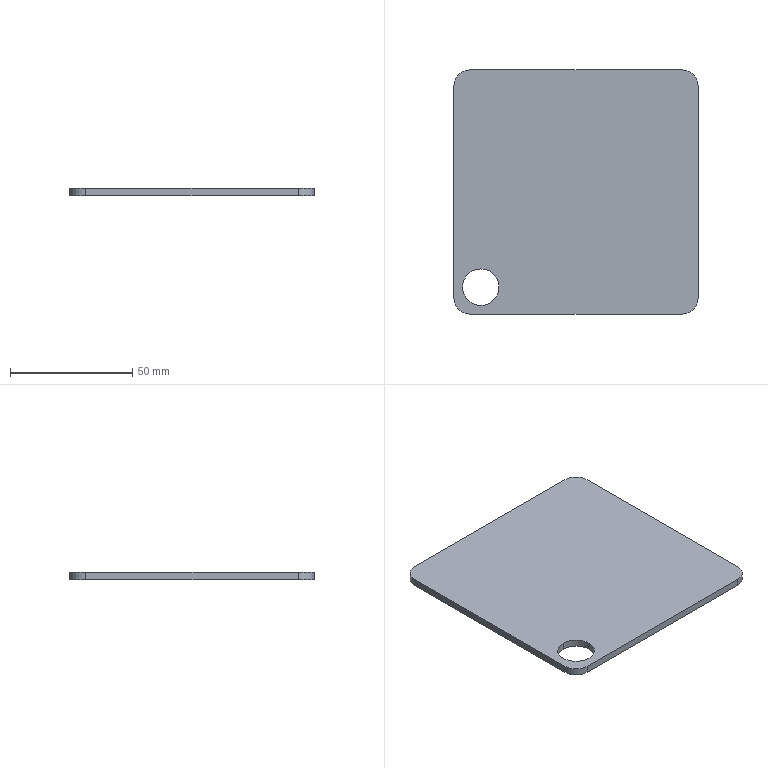Part | STEP file | [14] | 1 solid | 12 faces | box 100 x 100 x 3 mm | volume 29364 mm3 | cylinder 6 | plane 6 | commonest cylinder face diameters 12.8 x4 15 x2
STEP:
#1=CARTESIAN_POINT('',(0.,0.,0.));
#2=DIRECTION('',(0.,0.,1.));
#3=DIRECTION('',(1.,0.,0.));
#4=AXIS2_PLACEMENT_3D('',#1,#2,#3);
#5=CARTESIAN_POINT('',(11.,3.5,0.));
#6=VERTEX_POINT('',#5);
#7=CARTESIAN_POINT('',(11.,3.5,3.));
#8=VERTEX_POINT('',#7);
#9=CARTESIAN_POINT('',(11.,3.5,0.));
#10=DIRECTION('',(0.,0.,1.));
#11=VECTOR('',#10,1.);
#12=LINE('',#9,#11);
#13=CARTESIAN_POINT('',(11.,11.,0.));
#14=DIRECTION('',(0.,0.,1.));
#15=DIRECTION('',(0.,-1.,0.));
#16=AXIS2_PLACEMENT_3D('',#13,#14,#15);
#17=CYLINDRICAL_SURFACE('',#16,7.5);
#18=CARTESIAN_POINT('',(6.283,0.));
#19=DIRECTION('',(0.,1.));
#20=VECTOR('',#19,1.);
#21=LINE('',#18,#20);
#22=(GEOMETRIC_REPRESENTATION_CONTEXT(2)PARAMETRIC_REPRESENTATION_CONTEXT()REPRESENTATION_CONTEXT('',''));
#23=DEFINITIONAL_REPRESENTATION('',(#21),#22);
#24=PCURVE('',#17,#23);
#25=CARTESIAN_POINT('',(11.,11.,0.));
#26=DIRECTION('',(0.,0.,1.));
#27=DIRECTION('',(0.,-1.,0.));
#28=AXIS2_PLACEMENT_3D('',#25,#26,#27);
#29=CYLINDRICAL_SURFACE('',#28,7.5);
#30=CARTESIAN_POINT('',(0.,0.));
#31=DIRECTION('',(0.,1.));
#32=VECTOR('',#31,1.);
#33=LINE('',#30,#32);
#34=(GEOMETRIC_REPRESENTATION_CONTEXT(2)PARAMETRIC_REPRESENTATION_CONTEXT()REPRESENTATION_CONTEXT('',''));
#35=DEFINITIONAL_REPRESENTATION('',(#33),#34);
#36=PCURVE('',#29,#35);
#37=SURFACE_CURVE('',#12,(#24,#36),.PCURVE_S1.);
#38=EDGE_CURVE('',#6,#8,#37,.T.);
#39=ORIENTED_EDGE('',*,*,#38,.T.);
#40=CARTESIAN_POINT('',(11.,18.5,3.));
#41=VERTEX_POINT('',#40);
#42=CARTESIAN_POINT('',(11.,11.,3.));
#43=DIRECTION('',(0.,0.,-1.));
#44=DIRECTION('',(0.,1.,0.));
#45=AXIS2_PLACEMENT_3D('',#42,#43,#44);
#46=CIRCLE('',#45,7.5);
#47=CARTESIAN_POINT('',(9.425,3.));
#48=DIRECTION('',(-1.,0.));
#49=VECTOR('',#48,1.);
#50=LINE('',#47,#49);
#51=(GEOMETRIC_REPRESENTATION_CONTEXT(2)PARAMETRIC_REPRESENTATION_CONTEXT()REPRESENTATION_CONTEXT('',''));
#52=DEFINITIONAL_REPRESENTATION('',(#50),#51);
#53=PCURVE('',#17,#52);
#54=CARTESIAN_POINT('',(50.,50.,3.));
#55=DIRECTION('',(0.,0.,1.));
#56=DIRECTION('',(-1.,0.,0.));
#57=AXIS2_PLACEMENT_3D('',#54,#55,#56);
#58=PLANE('',#57);
#59=CARTESIAN_POINT('',(39.,31.5));
#60=CARTESIAN_POINT('',(26.01,31.5));
#61=CARTESIAN_POINT('',(32.505,42.75));
#62=CARTESIAN_POINT('',(39.,54.));
#63=CARTESIAN_POINT('',(45.495,42.75));
#64=CARTESIAN_POINT('',(51.99,31.5));
#65=CARTESIAN_POINT('',(39.,31.5));
#66=(BOUNDED_CURVE()B_SPLINE_CURVE(2,(#59,#60,#61,#62,#63,#64,#65),.UNSPECIFIED.,.T.,.F.)B_SPLINE_CURVE_WITH_KNOTS((1,2,2,2,2,1),(-2.094,0.,2.094,4.189,6.283,8.378),.UNSPECIFIED.)CURVE()GEOMETRIC_REPRESENTATION_ITEM()RATIONAL_B_SPLINE_CURVE((1.,0.5,1.,0.5,1.,0.5,1.))REPRESENTATION_ITEM(''));
#67=(GEOMETRIC_REPRESENTATION_CONTEXT(2)PARAMETRIC_REPRESENTATION_CONTEXT()REPRESENTATION_CONTEXT('',''));
#68=DEFINITIONAL_REPRESENTATION('',(#66),#67);
#69=PCURVE('',#58,#68);
#70=SURFACE_CURVE('',#46,(#53,#69),.PCURVE_S1.);
#71=EDGE_CURVE('',#8,#41,#70,.T.);
#72=ORIENTED_EDGE('',*,*,#71,.T.);
#73=CARTESIAN_POINT('',(11.,18.5,0.));
#74=VERTEX_POINT('',#73);
#75=CARTESIAN_POINT('',(11.,18.5,0.));
#76=DIRECTION('',(0.,0.,1.));
#77=VECTOR('',#76,1.);
#78=LINE('',#75,#77);
#79=CARTESIAN_POINT('',(3.142,0.));
#80=DIRECTION('',(0.,1.));
#81=VECTOR('',#80,1.);
#82=LINE('',#79,#81);
#83=(GEOMETRIC_REPRESENTATION_CONTEXT(2)PARAMETRIC_REPRESENTATION_CONTEXT()REPRESENTATION_CONTEXT('',''));
#84=DEFINITIONAL_REPRESENTATION('',(#82),#83);
#85=PCURVE('',#17,#84);
#86=CARTESIAN_POINT('',(3.142,0.));
#87=DIRECTION('',(0.,1.));
#88=VECTOR('',#87,1.);
#89=LINE('',#86,#88);
#90=(GEOMETRIC_REPRESENTATION_CONTEXT(2)PARAMETRIC_REPRESENTATION_CONTEXT()REPRESENTATION_CONTEXT('',''));
#91=DEFINITIONAL_REPRESENTATION('',(#89),#90);
#92=PCURVE('',#29,#91);
#93=SURFACE_CURVE('',#78,(#85,#92),.PCURVE_S1.);
#94=EDGE_CURVE('',#74,#41,#93,.T.);
#95=ORIENTED_EDGE('',*,*,#94,.F.);
#96=CARTESIAN_POINT('',(11.,11.,0.));
#97=DIRECTION('',(0.,0.,1.));
#98=DIRECTION('',(0.,-1.,0.));
#99=AXIS2_PLACEMENT_3D('',#96,#97,#98);
#100=CIRCLE('',#99,7.5);
#101=CARTESIAN_POINT('',(0.,0.));
#102=DIRECTION('',(1.,0.));
#103=VECTOR('',#102,1.);
#104=LINE('',#101,#103);
#105=(GEOMETRIC_REPRESENTATION_CONTEXT(2)PARAMETRIC_REPRESENTATION_CONTEXT()REPRESENTATION_CONTEXT('',''));
#106=DEFINITIONAL_REPRESENTATION('',(#104),#105);
#107=PCURVE('',#17,#106);
#108=CARTESIAN_POINT('',(50.,50.,0.));
#109=DIRECTION('',(0.,0.,-1.));
#110=DIRECTION('',(1.,0.,0.));
#111=AXIS2_PLACEMENT_3D('',#108,#109,#110);
#112=PLANE('',#111);
#113=CARTESIAN_POINT('',(-39.,46.5));
#114=CARTESIAN_POINT('',(-26.01,46.5));
#115=CARTESIAN_POINT('',(-32.505,35.25));
#116=CARTESIAN_POINT('',(-39.,24.));
#117=CARTESIAN_POINT('',(-45.495,35.25));
#118=CARTESIAN_POINT('',(-51.99,46.5));
#119=CARTESIAN_POINT('',(-39.,46.5));
#120=(BOUNDED_CURVE()B_SPLINE_CURVE(2,(#113,#114,#115,#116,#117,#118,#119),.UNSPECIFIED.,.T.,.F.)B_SPLINE_CURVE_WITH_KNOTS((1,2,2,2,2,1),(-2.094,0.,2.094,4.189,6.283,8.378),.UNSPECIFIED.)CURVE()GEOMETRIC_REPRESENTATION_ITEM()RATIONAL_B_SPLINE_CURVE((1.,0.5,1.,0.5,1.,0.5,1.))REPRESENTATION_ITEM(''));
#121=(GEOMETRIC_REPRESENTATION_CONTEXT(2)PARAMETRIC_REPRESENTATION_CONTEXT()REPRESENTATION_CONTEXT('',''));
#122=DEFINITIONAL_REPRESENTATION('',(#120),#121);
#123=PCURVE('',#112,#122);
#124=SURFACE_CURVE('',#100,(#107,#123),.PCURVE_S1.);
#125=EDGE_CURVE('',#74,#6,#124,.T.);
#126=ORIENTED_EDGE('',*,*,#125,.T.);
#127=EDGE_LOOP('',(#39,#72,#95,#126));
#128=FACE_BOUND('',#127,.F.);
#129=ADVANCED_FACE('',(#128),#17,.F.);
#130=CARTESIAN_POINT('',(11.,11.,0.));
#131=DIRECTION('',(0.,0.,1.));
#132=DIRECTION('',(0.,-1.,0.));
#133=AXIS2_PLACEMENT_3D('',#130,#131,#132);
#134=CIRCLE('',#133,7.5);
#135=CARTESIAN_POINT('',(-39.,46.5));
#136=CARTESIAN_POINT('',(-26.01,46.5));
#137=CARTESIAN_POINT('',(-32.505,35.25));
#138=CARTESIAN_POINT('',(-39.,24.));
#139=CARTESIAN_POINT('',(-45.495,35.25));
#140=CARTESIAN_POINT('',(-51.99,46.5));
#141=CARTESIAN_POINT('',(-39.,46.5));
#142=(BOUNDED_CURVE()B_SPLINE_CURVE(2,(#135,#136,#137,#138,#139,#140,#141),.UNSPECIFIED.,.T.,.F.)B_SPLINE_CURVE_WITH_KNOTS((1,2,2,2,2,1),(-2.094,0.,2.094,4.189,6.283,8.378),.UNSPECIFIED.)CURVE()GEOMETRIC_REPRESENTATION_ITEM()RATIONAL_B_SPLINE_CURVE((1.,0.5,1.,0.5,1.,0.5,1.))REPRESENTATION_ITEM(''));
#143=(GEOMETRIC_REPRESENTATION_CONTEXT(2)PARAMETRIC_REPRESENTATION_CONTEXT()REPRESENTATION_CONTEXT('',''));
#144=DEFINITIONAL_REPRESENTATION('',(#142),#143);
#145=PCURVE('',#112,#144);
#146=CARTESIAN_POINT('',(0.,0.));
#147=DIRECTION('',(1.,0.));
#148=VECTOR('',#147,1.);
#149=LINE('',#146,#148);
#150=(GEOMETRIC_REPRESENTATION_CONTEXT(2)PARAMETRIC_REPRESENTATION_CONTEXT()REPRESENTATION_CONTEXT('',''));
#151=DEFINITIONAL_REPRESENTATION('',(#149),#150);
#152=PCURVE('',#29,#151);
#153=SURFACE_CURVE('',#134,(#145,#152),.PCURVE_S1.);
#154=EDGE_CURVE('',#6,#74,#153,.T.);
#155=ORIENTED_EDGE('',*,*,#154,.T.);
#156=ORIENTED_EDGE('',*,*,#125,.T.);
#157=EDGE_LOOP('',(#155,#156));
#158=FACE_BOUND('',#157,.T.);
#159=CARTESIAN_POINT('',(0.,93.6,0.));
#160=VERTEX_POINT('',#159);
#161=CARTESIAN_POINT('',(0.,6.4,0.));
#162=VERTEX_POINT('',#161);
#163=CARTESIAN_POINT('',(0.,50.,0.));
#164=DIRECTION('',(0.,-1.,0.));
#165=VECTOR('',#164,1.);
#166=LINE('',#163,#165);
#167=CARTESIAN_POINT('',(-50.,0.));
#168=DIRECTION('',(0.,1.));
#169=VECTOR('',#168,1.);
#170=LINE('',#167,#169);
#171=(GEOMETRIC_REPRESENTATION_CONTEXT(2)PARAMETRIC_REPRESENTATION_CONTEXT()REPRESENTATION_CONTEXT('',''));
#172=DEFINITIONAL_REPRESENTATION('',(#170),#171);
#173=PCURVE('',#112,#172);
#174=CARTESIAN_POINT('',(0.,50.,3.));
#175=DIRECTION('',(-1.,0.,0.));
#176=DIRECTION('',(0.,0.,-1.));
#177=AXIS2_PLACEMENT_3D('',#174,#175,#176);
#178=PLANE('',#177);
#179=CARTESIAN_POINT('',(3.,0.));
#180=DIRECTION('',(0.,1.));
#181=VECTOR('',#180,1.);
#182=LINE('',#179,#181);
#183=(GEOMETRIC_REPRESENTATION_CONTEXT(2)PARAMETRIC_REPRESENTATION_CONTEXT()REPRESENTATION_CONTEXT('',''));
#184=DEFINITIONAL_REPRESENTATION('',(#182),#183);
#185=PCURVE('',#178,#184);
#186=SURFACE_CURVE('',#166,(#173,#185),.PCURVE_S1.);
#187=EDGE_CURVE('',#160,#162,#186,.T.);
#188=ORIENTED_EDGE('',*,*,#187,.F.);
#189=CARTESIAN_POINT('',(6.4,100.,0.));
#190=VERTEX_POINT('',#189);
#191=CARTESIAN_POINT('',(6.4,93.6,0.));
#192=DIRECTION('',(0.,0.,-1.));
#193=DIRECTION('',(1.,0.,0.));
#194=AXIS2_PLACEMENT_3D('',#191,#192,#193);
#195=CIRCLE('',#194,6.4);
#196=CARTESIAN_POINT('',(-43.6,-43.6));
#197=DIRECTION('',(1.,0.));
#198=AXIS2_PLACEMENT_2D('',#196,#197);
#199=CIRCLE('',#198,6.4);
#200=(GEOMETRIC_REPRESENTATION_CONTEXT(2)PARAMETRIC_REPRESENTATION_CONTEXT()REPRESENTATION_CONTEXT('',''));
#201=DEFINITIONAL_REPRESENTATION('',(#199),#200);
#202=PCURVE('',#112,#201);
#203=CARTESIAN_POINT('',(6.4,93.6,3.));
#204=DIRECTION('',(0.,0.,-1.));
#205=DIRECTION('',(1.,0.,0.));
#206=AXIS2_PLACEMENT_3D('',#203,#204,#205);
#207=CYLINDRICAL_SURFACE('',#206,6.4);
#208=CARTESIAN_POINT('',(0.,3.));
#209=DIRECTION('',(1.,0.));
#210=VECTOR('',#209,1.);
#211=LINE('',#208,#210);
#212=(GEOMETRIC_REPRESENTATION_CONTEXT(2)PARAMETRIC_REPRESENTATION_CONTEXT()REPRESENTATION_CONTEXT('',''));
#213=DEFINITIONAL_REPRESENTATION('',(#211),#212);
#214=PCURVE('',#207,#213);
#215=SURFACE_CURVE('',#195,(#202,#214),.PCURVE_S1.);
#216=EDGE_CURVE('',#160,#190,#215,.T.);
#217=ORIENTED_EDGE('',*,*,#216,.T.);
#218=CARTESIAN_POINT('',(93.6,100.,0.));
#219=VERTEX_POINT('',#218);
#220=CARTESIAN_POINT('',(50.,100.,0.));
#221=DIRECTION('',(-1.,0.,0.));
#222=VECTOR('',#221,1.);
#223=LINE('',#220,#222);
#224=CARTESIAN_POINT('',(0.,-50.));
#225=DIRECTION('',(-1.,0.));
#226=VECTOR('',#225,1.);
#227=LINE('',#224,#226);
#228=(GEOMETRIC_REPRESENTATION_CONTEXT(2)PARAMETRIC_REPRESENTATION_CONTEXT()REPRESENTATION_CONTEXT('',''));
#229=DEFINITIONAL_REPRESENTATION('',(#227),#228);
#230=PCURVE('',#112,#229);
#231=CARTESIAN_POINT('',(50.,100.,3.));
#232=DIRECTION('',(0.,1.,0.));
#233=DIRECTION('',(0.,0.,1.));
#234=AXIS2_PLACEMENT_3D('',#231,#232,#233);
#235=PLANE('',#234);
#236=CARTESIAN_POINT('',(-3.,0.));
#237=DIRECTION('',(0.,-1.));
#238=VECTOR('',#237,1.);
#239=LINE('',#236,#238);
#240=(GEOMETRIC_REPRESENTATION_CONTEXT(2)PARAMETRIC_REPRESENTATION_CONTEXT()REPRESENTATION_CONTEXT('',''));
#241=DEFINITIONAL_REPRESENTATION('',(#239),#240);
#242=PCURVE('',#235,#241);
#243=SURFACE_CURVE('',#223,(#230,#242),.PCURVE_S1.);
#244=EDGE_CURVE('',#219,#190,#243,.T.);
#245=ORIENTED_EDGE('',*,*,#244,.F.);
#246=CARTESIAN_POINT('',(100.,93.6,0.));
#247=VERTEX_POINT('',#246);
#248=CARTESIAN_POINT('',(93.6,93.6,0.));
#249=DIRECTION('',(0.,0.,-1.));
#250=DIRECTION('',(1.,0.,0.));
#251=AXIS2_PLACEMENT_3D('',#248,#249,#250);
#252=CIRCLE('',#251,6.4);
#253=CARTESIAN_POINT('',(43.6,-43.6));
#254=DIRECTION('',(1.,0.));
#255=AXIS2_PLACEMENT_2D('',#253,#254);
#256=CIRCLE('',#255,6.4);
#257=(GEOMETRIC_REPRESENTATION_CONTEXT(2)PARAMETRIC_REPRESENTATION_CONTEXT()REPRESENTATION_CONTEXT('',''));
#258=DEFINITIONAL_REPRESENTATION('',(#256),#257);
#259=PCURVE('',#112,#258);
#260=CARTESIAN_POINT('',(93.6,93.6,3.));
#261=DIRECTION('',(0.,0.,-1.));
#262=DIRECTION('',(1.,0.,0.));
#263=AXIS2_PLACEMENT_3D('',#260,#261,#262);
#264=CYLINDRICAL_SURFACE('',#263,6.4);
#265=CARTESIAN_POINT('',(0.,3.));
#266=DIRECTION('',(1.,0.));
#267=VECTOR('',#266,1.);
#268=LINE('',#265,#267);
#269=(GEOMETRIC_REPRESENTATION_CONTEXT(2)PARAMETRIC_REPRESENTATION_CONTEXT()REPRESENTATION_CONTEXT('',''));
#270=DEFINITIONAL_REPRESENTATION('',(#268),#269);
#271=PCURVE('',#264,#270);
#272=SURFACE_CURVE('',#252,(#259,#271),.PCURVE_S1.);
#273=EDGE_CURVE('',#219,#247,#272,.T.);
#274=ORIENTED_EDGE('',*,*,#273,.T.);
#275=CARTESIAN_POINT('',(100.,6.4,0.));
#276=VERTEX_POINT('',#275);
#277=CARTESIAN_POINT('',(100.,50.,0.));
#278=DIRECTION('',(0.,1.,0.));
#279=VECTOR('',#278,1.);
#280=LINE('',#277,#279);
#281=CARTESIAN_POINT('',(50.,0.));
#282=DIRECTION('',(0.,-1.));
#283=VECTOR('',#282,1.);
#284=LINE('',#281,#283);
#285=(GEOMETRIC_REPRESENTATION_CONTEXT(2)PARAMETRIC_REPRESENTATION_CONTEXT()REPRESENTATION_CONTEXT('',''));
#286=DEFINITIONAL_REPRESENTATION('',(#284),#285);
#287=PCURVE('',#112,#286);
#288=CARTESIAN_POINT('',(100.,50.,3.));
#289=DIRECTION('',(1.,0.,0.));
#290=DIRECTION('',(0.,0.,1.));
#291=AXIS2_PLACEMENT_3D('',#288,#289,#290);
#292=PLANE('',#291);
#293=CARTESIAN_POINT('',(-3.,0.));
#294=DIRECTION('',(0.,-1.));
#295=VECTOR('',#294,1.);
#296=LINE('',#293,#295);
#297=(GEOMETRIC_REPRESENTATION_CONTEXT(2)PARAMETRIC_REPRESENTATION_CONTEXT()REPRESENTATION_CONTEXT('',''));
#298=DEFINITIONAL_REPRESENTATION('',(#296),#297);
#299=PCURVE('',#292,#298);
#300=SURFACE_CURVE('',#280,(#287,#299),.PCURVE_S1.);
#301=EDGE_CURVE('',#276,#247,#300,.T.);
#302=ORIENTED_EDGE('',*,*,#301,.F.);
#303=CARTESIAN_POINT('',(93.6,0.,0.));
#304=VERTEX_POINT('',#303);
#305=CARTESIAN_POINT('',(93.6,6.4,0.));
#306=DIRECTION('',(0.,0.,-1.));
#307=DIRECTION('',(1.,0.,0.));
#308=AXIS2_PLACEMENT_3D('',#305,#306,#307);
#309=CIRCLE('',#308,6.4);
#310=CARTESIAN_POINT('',(43.6,43.6));
#311=DIRECTION('',(1.,0.));
#312=AXIS2_PLACEMENT_2D('',#310,#311);
#313=CIRCLE('',#312,6.4);
#314=(GEOMETRIC_REPRESENTATION_CONTEXT(2)PARAMETRIC_REPRESENTATION_CONTEXT()REPRESENTATION_CONTEXT('',''));
#315=DEFINITIONAL_REPRESENTATION('',(#313),#314);
#316=PCURVE('',#112,#315);
#317=CARTESIAN_POINT('',(93.6,6.4,3.));
#318=DIRECTION('',(0.,0.,-1.));
#319=DIRECTION('',(1.,0.,0.));
#320=AXIS2_PLACEMENT_3D('',#317,#318,#319);
#321=CYLINDRICAL_SURFACE('',#320,6.4);
#322=CARTESIAN_POINT('',(0.,3.));
#323=DIRECTION('',(1.,0.));
#324=VECTOR('',#323,1.);
#325=LINE('',#322,#324);
#326=(GEOMETRIC_REPRESENTATION_CONTEXT(2)PARAMETRIC_REPRESENTATION_CONTEXT()REPRESENTATION_CONTEXT('',''));
#327=DEFINITIONAL_REPRESENTATION('',(#325),#326);
#328=PCURVE('',#321,#327);
#329=SURFACE_CURVE('',#309,(#316,#328),.PCURVE_S1.);
#330=EDGE_CURVE('',#276,#304,#329,.T.);
#331=ORIENTED_EDGE('',*,*,#330,.T.);
#332=CARTESIAN_POINT('',(6.4,0.,0.));
#333=VERTEX_POINT('',#332);
#334=CARTESIAN_POINT('',(50.,0.,0.));
#335=DIRECTION('',(1.,0.,0.));
#336=VECTOR('',#335,1.);
#337=LINE('',#334,#336);
#338=CARTESIAN_POINT('',(0.,50.));
#339=DIRECTION('',(1.,0.));
#340=VECTOR('',#339,1.);
#341=LINE('',#338,#340);
#342=(GEOMETRIC_REPRESENTATION_CONTEXT(2)PARAMETRIC_REPRESENTATION_CONTEXT()REPRESENTATION_CONTEXT('',''));
#343=DEFINITIONAL_REPRESENTATION('',(#341),#342);
#344=PCURVE('',#112,#343);
#345=CARTESIAN_POINT('',(50.,0.,3.));
#346=DIRECTION('',(0.,-1.,0.));
#347=DIRECTION('',(0.,0.,-1.));
#348=AXIS2_PLACEMENT_3D('',#345,#346,#347);
#349=PLANE('',#348);
#350=CARTESIAN_POINT('',(3.,0.));
#351=DIRECTION('',(0.,1.));
#352=VECTOR('',#351,1.);
#353=LINE('',#350,#352);
#354=(GEOMETRIC_REPRESENTATION_CONTEXT(2)PARAMETRIC_REPRESENTATION_CONTEXT()REPRESENTATION_CONTEXT('',''));
#355=DEFINITIONAL_REPRESENTATION('',(#353),#354);
#356=PCURVE('',#349,#355);
#357=SURFACE_CURVE('',#337,(#344,#356),.PCURVE_S1.);
#358=EDGE_CURVE('',#333,#304,#357,.T.);
#359=ORIENTED_EDGE('',*,*,#358,.F.);
#360=CARTESIAN_POINT('',(6.4,6.4,0.));
#361=DIRECTION('',(0.,0.,-1.));
#362=DIRECTION('',(1.,0.,0.));
#363=AXIS2_PLACEMENT_3D('',#360,#361,#362);
#364=CIRCLE('',#363,6.4);
#365=CARTESIAN_POINT('',(-43.6,43.6));
#366=DIRECTION('',(1.,0.));
#367=AXIS2_PLACEMENT_2D('',#365,#366);
#368=CIRCLE('',#367,6.4);
#369=(GEOMETRIC_REPRESENTATION_CONTEXT(2)PARAMETRIC_REPRESENTATION_CONTEXT()REPRESENTATION_CONTEXT('',''));
#370=DEFINITIONAL_REPRESENTATION('',(#368),#369);
#371=PCURVE('',#112,#370);
#372=CARTESIAN_POINT('',(6.4,6.4,3.));
#373=DIRECTION('',(0.,0.,-1.));
#374=DIRECTION('',(1.,0.,0.));
#375=AXIS2_PLACEMENT_3D('',#372,#373,#374);
#376=CYLINDRICAL_SURFACE('',#375,6.4);
#377=CARTESIAN_POINT('',(0.,3.));
#378=DIRECTION('',(1.,0.));
#379=VECTOR('',#378,1.);
#380=LINE('',#377,#379);
#381=(GEOMETRIC_REPRESENTATION_CONTEXT(2)PARAMETRIC_REPRESENTATION_CONTEXT()REPRESENTATION_CONTEXT('',''));
#382=DEFINITIONAL_REPRESENTATION('',(#380),#381);
#383=PCURVE('',#376,#382);
#384=SURFACE_CURVE('',#364,(#371,#383),.PCURVE_S1.);
#385=EDGE_CURVE('',#333,#162,#384,.T.);
#386=ORIENTED_EDGE('',*,*,#385,.T.);
#387=EDGE_LOOP('',(#188,#217,#245,#274,#302,#331,#359,#386));
#388=FACE_BOUND('',#387,.T.);
#389=ADVANCED_FACE('',(#158,#388),#112,.T.);
#390=ORIENTED_EDGE('',*,*,#244,.T.);
#391=CARTESIAN_POINT('',(6.4,100.,3.));
#392=VERTEX_POINT('',#391);
#393=CARTESIAN_POINT('',(6.4,100.,3.));
#394=DIRECTION('',(0.,0.,1.));
#395=VECTOR('',#394,1.);
#396=LINE('',#393,#395);
#397=CARTESIAN_POINT('',(0.,-43.6));
#398=DIRECTION('',(1.,0.));
#399=VECTOR('',#398,1.);
#400=LINE('',#397,#399);
#401=(GEOMETRIC_REPRESENTATION_CONTEXT(2)PARAMETRIC_REPRESENTATION_CONTEXT()REPRESENTATION_CONTEXT('',''));
#402=DEFINITIONAL_REPRESENTATION('',(#400),#401);
#403=PCURVE('',#235,#402);
#404=CARTESIAN_POINT('',(4.712,0.));
#405=DIRECTION('',(0.,-1.));
#406=VECTOR('',#405,1.);
#407=LINE('',#404,#406);
#408=(GEOMETRIC_REPRESENTATION_CONTEXT(2)PARAMETRIC_REPRESENTATION_CONTEXT()REPRESENTATION_CONTEXT('',''));
#409=DEFINITIONAL_REPRESENTATION('',(#407),#408);
#410=PCURVE('',#207,#409);
#411=SURFACE_CURVE('',#396,(#403,#410),.PCURVE_S1.);
#412=EDGE_CURVE('',#190,#392,#411,.T.);
#413=ORIENTED_EDGE('',*,*,#412,.T.);
#414=CARTESIAN_POINT('',(93.6,100.,3.));
#415=VERTEX_POINT('',#414);
#416=CARTESIAN_POINT('',(50.,100.,3.));
#417=DIRECTION('',(1.,0.,0.));
#418=VECTOR('',#417,1.);
#419=LINE('',#416,#418);
#420=CARTESIAN_POINT('',(0.,0.));
#421=DIRECTION('',(0.,1.));
#422=VECTOR('',#421,1.);
#423=LINE('',#420,#422);
#424=(GEOMETRIC_REPRESENTATION_CONTEXT(2)PARAMETRIC_REPRESENTATION_CONTEXT()REPRESENTATION_CONTEXT('',''));
#425=DEFINITIONAL_REPRESENTATION('',(#423),#424);
#426=PCURVE('',#235,#425);
#427=CARTESIAN_POINT('',(0.,-50.));
#428=DIRECTION('',(-1.,0.));
#429=VECTOR('',#428,1.);
#430=LINE('',#427,#429);
#431=(GEOMETRIC_REPRESENTATION_CONTEXT(2)PARAMETRIC_REPRESENTATION_CONTEXT()REPRESENTATION_CONTEXT('',''));
#432=DEFINITIONAL_REPRESENTATION('',(#430),#431);
#433=PCURVE('',#58,#432);
#434=SURFACE_CURVE('',#419,(#426,#433),.PCURVE_S1.);
#435=EDGE_CURVE('',#392,#415,#434,.T.);
#436=ORIENTED_EDGE('',*,*,#435,.T.);
#437=CARTESIAN_POINT('',(93.6,100.,3.));
#438=DIRECTION('',(0.,0.,-1.));
#439=VECTOR('',#438,1.);
#440=LINE('',#437,#439);
#441=CARTESIAN_POINT('',(0.,43.6));
#442=DIRECTION('',(-1.,0.));
#443=VECTOR('',#442,1.);
#444=LINE('',#441,#443);
#445=(GEOMETRIC_REPRESENTATION_CONTEXT(2)PARAMETRIC_REPRESENTATION_CONTEXT()REPRESENTATION_CONTEXT('',''));
#446=DEFINITIONAL_REPRESENTATION('',(#444),#445);
#447=PCURVE('',#235,#446);
#448=CARTESIAN_POINT('',(4.712,0.));
#449=DIRECTION('',(0.,1.));
#450=VECTOR('',#449,1.);
#451=LINE('',#448,#450);
#452=(GEOMETRIC_REPRESENTATION_CONTEXT(2)PARAMETRIC_REPRESENTATION_CONTEXT()REPRESENTATION_CONTEXT('',''));
#453=DEFINITIONAL_REPRESENTATION('',(#451),#452);
#454=PCURVE('',#264,#453);
#455=SURFACE_CURVE('',#440,(#447,#454),.PCURVE_S1.);
#456=EDGE_CURVE('',#415,#219,#455,.T.);
#457=ORIENTED_EDGE('',*,*,#456,.T.);
#458=EDGE_LOOP('',(#390,#413,#436,#457));
#459=FACE_BOUND('',#458,.T.);
#460=ADVANCED_FACE('',(#459),#235,.T.);
#461=CARTESIAN_POINT('',(0.,6.4,3.));
#462=VERTEX_POINT('',#461);
#463=CARTESIAN_POINT('',(0.,93.6,3.));
#464=VERTEX_POINT('',#463);
#465=CARTESIAN_POINT('',(0.,50.,3.));
#466=DIRECTION('',(0.,1.,0.));
#467=VECTOR('',#466,1.);
#468=LINE('',#465,#467);
#469=CARTESIAN_POINT('',(0.,0.));
#470=DIRECTION('',(0.,-1.));
#471=VECTOR('',#470,1.);
#472=LINE('',#469,#471);
#473=(GEOMETRIC_REPRESENTATION_CONTEXT(2)PARAMETRIC_REPRESENTATION_CONTEXT()REPRESENTATION_CONTEXT('',''));
#474=DEFINITIONAL_REPRESENTATION('',(#472),#473);
#475=PCURVE('',#178,#474);
#476=CARTESIAN_POINT('',(50.,0.));
#477=DIRECTION('',(0.,-1.));
#478=VECTOR('',#477,1.);
#479=LINE('',#476,#478);
#480=(GEOMETRIC_REPRESENTATION_CONTEXT(2)PARAMETRIC_REPRESENTATION_CONTEXT()REPRESENTATION_CONTEXT('',''));
#481=DEFINITIONAL_REPRESENTATION('',(#479),#480);
#482=PCURVE('',#58,#481);
#483=SURFACE_CURVE('',#468,(#475,#482),.PCURVE_S1.);
#484=EDGE_CURVE('',#462,#464,#483,.T.);
#485=ORIENTED_EDGE('',*,*,#484,.T.);
#486=CARTESIAN_POINT('',(0.,93.6,3.));
#487=DIRECTION('',(0.,0.,-1.));
#488=VECTOR('',#487,1.);
#489=LINE('',#486,#488);
#490=CARTESIAN_POINT('',(0.,-43.6));
#491=DIRECTION('',(1.,0.));
#492=VECTOR('',#491,1.);
#493=LINE('',#490,#492);
#494=(GEOMETRIC_REPRESENTATION_CONTEXT(2)PARAMETRIC_REPRESENTATION_CONTEXT()REPRESENTATION_CONTEXT('',''));
#495=DEFINITIONAL_REPRESENTATION('',(#493),#494);
#496=PCURVE('',#178,#495);
#497=CARTESIAN_POINT('',(3.142,0.));
#498=DIRECTION('',(0.,1.));
#499=VECTOR('',#498,1.);
#500=LINE('',#497,#499);
#501=(GEOMETRIC_REPRESENTATION_CONTEXT(2)PARAMETRIC_REPRESENTATION_CONTEXT()REPRESENTATION_CONTEXT('',''));
#502=DEFINITIONAL_REPRESENTATION('',(#500),#501);
#503=PCURVE('',#207,#502);
#504=SURFACE_CURVE('',#489,(#496,#503),.PCURVE_S1.);
#505=EDGE_CURVE('',#464,#160,#504,.T.);
#506=ORIENTED_EDGE('',*,*,#505,.T.);
#507=ORIENTED_EDGE('',*,*,#187,.T.);
#508=CARTESIAN_POINT('',(0.,6.4,3.));
#509=DIRECTION('',(0.,0.,1.));
#510=VECTOR('',#509,1.);
#511=LINE('',#508,#510);
#512=CARTESIAN_POINT('',(0.,43.6));
#513=DIRECTION('',(-1.,0.));
#514=VECTOR('',#513,1.);
#515=LINE('',#512,#514);
#516=(GEOMETRIC_REPRESENTATION_CONTEXT(2)PARAMETRIC_REPRESENTATION_CONTEXT()REPRESENTATION_CONTEXT('',''));
#517=DEFINITIONAL_REPRESENTATION('',(#515),#516);
#518=PCURVE('',#178,#517);
#519=CARTESIAN_POINT('',(3.142,0.));
#520=DIRECTION('',(0.,-1.));
#521=VECTOR('',#520,1.);
#522=LINE('',#519,#521);
#523=(GEOMETRIC_REPRESENTATION_CONTEXT(2)PARAMETRIC_REPRESENTATION_CONTEXT()REPRESENTATION_CONTEXT('',''));
#524=DEFINITIONAL_REPRESENTATION('',(#522),#523);
#525=PCURVE('',#376,#524);
#526=SURFACE_CURVE('',#511,(#518,#525),.PCURVE_S1.);
#527=EDGE_CURVE('',#162,#462,#526,.T.);
#528=ORIENTED_EDGE('',*,*,#527,.T.);
#529=EDGE_LOOP('',(#485,#506,#507,#528));
#530=FACE_BOUND('',#529,.T.);
#531=ADVANCED_FACE('',(#530),#178,.T.);
#532=ORIENTED_EDGE('',*,*,#358,.T.);
#533=CARTESIAN_POINT('',(93.6,0.,3.));
#534=VERTEX_POINT('',#533);
#535=CARTESIAN_POINT('',(93.6,0.,3.));
#536=DIRECTION('',(0.,0.,1.));
#537=VECTOR('',#536,1.);
#538=LINE('',#535,#537);
#539=CARTESIAN_POINT('',(0.,43.6));
#540=DIRECTION('',(-1.,0.));
#541=VECTOR('',#540,1.);
#542=LINE('',#539,#541);
#543=(GEOMETRIC_REPRESENTATION_CONTEXT(2)PARAMETRIC_REPRESENTATION_CONTEXT()REPRESENTATION_CONTEXT('',''));
#544=DEFINITIONAL_REPRESENTATION('',(#542),#543);
#545=PCURVE('',#349,#544);
#546=CARTESIAN_POINT('',(1.571,0.));
#547=DIRECTION('',(0.,-1.));
#548=VECTOR('',#547,1.);
#549=LINE('',#546,#548);
#550=(GEOMETRIC_REPRESENTATION_CONTEXT(2)PARAMETRIC_REPRESENTATION_CONTEXT()REPRESENTATION_CONTEXT('',''));
#551=DEFINITIONAL_REPRESENTATION('',(#549),#550);
#552=PCURVE('',#321,#551);
#553=SURFACE_CURVE('',#538,(#545,#552),.PCURVE_S1.);
#554=EDGE_CURVE('',#304,#534,#553,.T.);
#555=ORIENTED_EDGE('',*,*,#554,.T.);
#556=CARTESIAN_POINT('',(6.4,0.,3.));
#557=VERTEX_POINT('',#556);
#558=CARTESIAN_POINT('',(50.,0.,3.));
#559=DIRECTION('',(-1.,0.,0.));
#560=VECTOR('',#559,1.);
#561=LINE('',#558,#560);
#562=CARTESIAN_POINT('',(0.,0.));
#563=DIRECTION('',(0.,-1.));
#564=VECTOR('',#563,1.);
#565=LINE('',#562,#564);
#566=(GEOMETRIC_REPRESENTATION_CONTEXT(2)PARAMETRIC_REPRESENTATION_CONTEXT()REPRESENTATION_CONTEXT('',''));
#567=DEFINITIONAL_REPRESENTATION('',(#565),#566);
#568=PCURVE('',#349,#567);
#569=CARTESIAN_POINT('',(0.,50.));
#570=DIRECTION('',(1.,0.));
#571=VECTOR('',#570,1.);
#572=LINE('',#569,#571);
#573=(GEOMETRIC_REPRESENTATION_CONTEXT(2)PARAMETRIC_REPRESENTATION_CONTEXT()REPRESENTATION_CONTEXT('',''));
#574=DEFINITIONAL_REPRESENTATION('',(#572),#573);
#575=PCURVE('',#58,#574);
#576=SURFACE_CURVE('',#561,(#568,#575),.PCURVE_S1.);
#577=EDGE_CURVE('',#534,#557,#576,.T.);
#578=ORIENTED_EDGE('',*,*,#577,.T.);
#579=CARTESIAN_POINT('',(6.4,0.,3.));
#580=DIRECTION('',(0.,0.,-1.));
#581=VECTOR('',#580,1.);
#582=LINE('',#579,#581);
#583=CARTESIAN_POINT('',(0.,-43.6));
#584=DIRECTION('',(1.,0.));
#585=VECTOR('',#584,1.);
#586=LINE('',#583,#585);
#587=(GEOMETRIC_REPRESENTATION_CONTEXT(2)PARAMETRIC_REPRESENTATION_CONTEXT()REPRESENTATION_CONTEXT('',''));
#588=DEFINITIONAL_REPRESENTATION('',(#586),#587);
#589=PCURVE('',#349,#588);
#590=CARTESIAN_POINT('',(1.571,0.));
#591=DIRECTION('',(0.,1.));
#592=VECTOR('',#591,1.);
#593=LINE('',#590,#592);
#594=(GEOMETRIC_REPRESENTATION_CONTEXT(2)PARAMETRIC_REPRESENTATION_CONTEXT()REPRESENTATION_CONTEXT('',''));
#595=DEFINITIONAL_REPRESENTATION('',(#593),#594);
#596=PCURVE('',#376,#595);
#597=SURFACE_CURVE('',#582,(#589,#596),.PCURVE_S1.);
#598=EDGE_CURVE('',#557,#333,#597,.T.);
#599=ORIENTED_EDGE('',*,*,#598,.T.);
#600=EDGE_LOOP('',(#532,#555,#578,#599));
#601=FACE_BOUND('',#600,.T.);
#602=ADVANCED_FACE('',(#601),#349,.T.);
#603=ORIENTED_EDGE('',*,*,#71,.T.);
#604=CARTESIAN_POINT('',(11.,11.,3.));
#605=DIRECTION('',(0.,0.,-1.));
#606=DIRECTION('',(0.,1.,0.));
#607=AXIS2_PLACEMENT_3D('',#604,#605,#606);
#608=CIRCLE('',#607,7.5);
#609=CARTESIAN_POINT('',(39.,31.5));
#610=CARTESIAN_POINT('',(26.01,31.5));
#611=CARTESIAN_POINT('',(32.505,42.75));
#612=CARTESIAN_POINT('',(39.,54.));
#613=CARTESIAN_POINT('',(45.495,42.75));
#614=CARTESIAN_POINT('',(51.99,31.5));
#615=CARTESIAN_POINT('',(39.,31.5));
#616=(BOUNDED_CURVE()B_SPLINE_CURVE(2,(#609,#610,#611,#612,#613,#614,#615),.UNSPECIFIED.,.T.,.F.)B_SPLINE_CURVE_WITH_KNOTS((1,2,2,2,2,1),(-2.094,0.,2.094,4.189,6.283,8.378),.UNSPECIFIED.)CURVE()GEOMETRIC_REPRESENTATION_ITEM()RATIONAL_B_SPLINE_CURVE((1.,0.5,1.,0.5,1.,0.5,1.))REPRESENTATION_ITEM(''));
#617=(GEOMETRIC_REPRESENTATION_CONTEXT(2)PARAMETRIC_REPRESENTATION_CONTEXT()REPRESENTATION_CONTEXT('',''));
#618=DEFINITIONAL_REPRESENTATION('',(#616),#617);
#619=PCURVE('',#58,#618);
#620=CARTESIAN_POINT('',(3.142,3.));
#621=DIRECTION('',(-1.,0.));
#622=VECTOR('',#621,1.);
#623=LINE('',#620,#622);
#624=(GEOMETRIC_REPRESENTATION_CONTEXT(2)PARAMETRIC_REPRESENTATION_CONTEXT()REPRESENTATION_CONTEXT('',''));
#625=DEFINITIONAL_REPRESENTATION('',(#623),#624);
#626=PCURVE('',#29,#625);
#627=SURFACE_CURVE('',#608,(#619,#626),.PCURVE_S1.);
#628=EDGE_CURVE('',#41,#8,#627,.T.);
#629=ORIENTED_EDGE('',*,*,#628,.T.);
#630=EDGE_LOOP('',(#603,#629));
#631=FACE_BOUND('',#630,.T.);
#632=ORIENTED_EDGE('',*,*,#435,.F.);
#633=CARTESIAN_POINT('',(6.4,93.6,3.));
#634=DIRECTION('',(0.,0.,1.));
#635=DIRECTION('',(-1.,0.,0.));
#636=AXIS2_PLACEMENT_3D('',#633,#634,#635);
#637=CIRCLE('',#636,6.4);
#638=CARTESIAN_POINT('',(43.6,-43.6));
#639=DIRECTION('',(1.,0.));
#640=AXIS2_PLACEMENT_2D('',#638,#639);
#641=CIRCLE('',#640,6.4);
#642=(GEOMETRIC_REPRESENTATION_CONTEXT(2)PARAMETRIC_REPRESENTATION_CONTEXT()REPRESENTATION_CONTEXT('',''));
#643=DEFINITIONAL_REPRESENTATION('',(#641),#642);
#644=PCURVE('',#58,#643);
#645=CARTESIAN_POINT('',(9.425,0.));
#646=DIRECTION('',(-1.,0.));
#647=VECTOR('',#646,1.);
#648=LINE('',#645,#647);
#649=(GEOMETRIC_REPRESENTATION_CONTEXT(2)PARAMETRIC_REPRESENTATION_CONTEXT()REPRESENTATION_CONTEXT('',''));
#650=DEFINITIONAL_REPRESENTATION('',(#648),#649);
#651=PCURVE('',#207,#650);
#652=SURFACE_CURVE('',#637,(#644,#651),.PCURVE_S1.);
#653=EDGE_CURVE('',#392,#464,#652,.T.);
#654=ORIENTED_EDGE('',*,*,#653,.T.);
#655=ORIENTED_EDGE('',*,*,#484,.F.);
#656=CARTESIAN_POINT('',(6.4,6.4,3.));
#657=DIRECTION('',(0.,0.,1.));
#658=DIRECTION('',(-1.,0.,0.));
#659=AXIS2_PLACEMENT_3D('',#656,#657,#658);
#660=CIRCLE('',#659,6.4);
#661=CARTESIAN_POINT('',(43.6,43.6));
#662=DIRECTION('',(1.,0.));
#663=AXIS2_PLACEMENT_2D('',#661,#662);
#664=CIRCLE('',#663,6.4);
#665=(GEOMETRIC_REPRESENTATION_CONTEXT(2)PARAMETRIC_REPRESENTATION_CONTEXT()REPRESENTATION_CONTEXT('',''));
#666=DEFINITIONAL_REPRESENTATION('',(#664),#665);
#667=PCURVE('',#58,#666);
#668=CARTESIAN_POINT('',(3.142,0.));
#669=DIRECTION('',(-1.,0.));
#670=VECTOR('',#669,1.);
#671=LINE('',#668,#670);
#672=(GEOMETRIC_REPRESENTATION_CONTEXT(2)PARAMETRIC_REPRESENTATION_CONTEXT()REPRESENTATION_CONTEXT('',''));
#673=DEFINITIONAL_REPRESENTATION('',(#671),#672);
#674=PCURVE('',#376,#673);
#675=SURFACE_CURVE('',#660,(#667,#674),.PCURVE_S1.);
#676=EDGE_CURVE('',#462,#557,#675,.T.);
#677=ORIENTED_EDGE('',*,*,#676,.T.);
#678=ORIENTED_EDGE('',*,*,#577,.F.);
#679=CARTESIAN_POINT('',(100.,6.4,3.));
#680=VERTEX_POINT('',#679);
#681=CARTESIAN_POINT('',(93.6,6.4,3.));
#682=DIRECTION('',(0.,0.,1.));
#683=DIRECTION('',(-1.,0.,0.));
#684=AXIS2_PLACEMENT_3D('',#681,#682,#683);
#685=CIRCLE('',#684,6.4);
#686=CARTESIAN_POINT('',(-43.6,43.6));
#687=DIRECTION('',(1.,0.));
#688=AXIS2_PLACEMENT_2D('',#686,#687);
#689=CIRCLE('',#688,6.4);
#690=(GEOMETRIC_REPRESENTATION_CONTEXT(2)PARAMETRIC_REPRESENTATION_CONTEXT()REPRESENTATION_CONTEXT('',''));
#691=DEFINITIONAL_REPRESENTATION('',(#689),#690);
#692=PCURVE('',#58,#691);
#693=CARTESIAN_POINT('',(3.142,0.));
#694=DIRECTION('',(-1.,0.));
#695=VECTOR('',#694,1.);
#696=LINE('',#693,#695);
#697=(GEOMETRIC_REPRESENTATION_CONTEXT(2)PARAMETRIC_REPRESENTATION_CONTEXT()REPRESENTATION_CONTEXT('',''));
#698=DEFINITIONAL_REPRESENTATION('',(#696),#697);
#699=PCURVE('',#321,#698);
#700=SURFACE_CURVE('',#685,(#692,#699),.PCURVE_S1.);
#701=EDGE_CURVE('',#534,#680,#700,.T.);
#702=ORIENTED_EDGE('',*,*,#701,.T.);
#703=CARTESIAN_POINT('',(100.,93.6,3.));
#704=VERTEX_POINT('',#703);
#705=CARTESIAN_POINT('',(100.,50.,3.));
#706=DIRECTION('',(0.,-1.,0.));
#707=VECTOR('',#706,1.);
#708=LINE('',#705,#707);
#709=CARTESIAN_POINT('',(-50.,0.));
#710=DIRECTION('',(0.,1.));
#711=VECTOR('',#710,1.);
#712=LINE('',#709,#711);
#713=(GEOMETRIC_REPRESENTATION_CONTEXT(2)PARAMETRIC_REPRESENTATION_CONTEXT()REPRESENTATION_CONTEXT('',''));
#714=DEFINITIONAL_REPRESENTATION('',(#712),#713);
#715=PCURVE('',#58,#714);
#716=CARTESIAN_POINT('',(0.,0.));
#717=DIRECTION('',(0.,1.));
#718=VECTOR('',#717,1.);
#719=LINE('',#716,#718);
#720=(GEOMETRIC_REPRESENTATION_CONTEXT(2)PARAMETRIC_REPRESENTATION_CONTEXT()REPRESENTATION_CONTEXT('',''));
#721=DEFINITIONAL_REPRESENTATION('',(#719),#720);
#722=PCURVE('',#292,#721);
#723=SURFACE_CURVE('',#708,(#715,#722),.PCURVE_S1.);
#724=EDGE_CURVE('',#704,#680,#723,.T.);
#725=ORIENTED_EDGE('',*,*,#724,.F.);
#726=CARTESIAN_POINT('',(93.6,93.6,3.));
#727=DIRECTION('',(0.,0.,1.));
#728=DIRECTION('',(-1.,0.,0.));
#729=AXIS2_PLACEMENT_3D('',#726,#727,#728);
#730=CIRCLE('',#729,6.4);
#731=CARTESIAN_POINT('',(-43.6,-43.6));
#732=DIRECTION('',(1.,0.));
#733=AXIS2_PLACEMENT_2D('',#731,#732);
#734=CIRCLE('',#733,6.4);
#735=(GEOMETRIC_REPRESENTATION_CONTEXT(2)PARAMETRIC_REPRESENTATION_CONTEXT()REPRESENTATION_CONTEXT('',''));
#736=DEFINITIONAL_REPRESENTATION('',(#734),#735);
#737=PCURVE('',#58,#736);
#738=CARTESIAN_POINT('',(9.425,0.));
#739=DIRECTION('',(-1.,0.));
#740=VECTOR('',#739,1.);
#741=LINE('',#738,#740);
#742=(GEOMETRIC_REPRESENTATION_CONTEXT(2)PARAMETRIC_REPRESENTATION_CONTEXT()REPRESENTATION_CONTEXT('',''));
#743=DEFINITIONAL_REPRESENTATION('',(#741),#742);
#744=PCURVE('',#264,#743);
#745=SURFACE_CURVE('',#730,(#737,#744),.PCURVE_S1.);
#746=EDGE_CURVE('',#704,#415,#745,.T.);
#747=ORIENTED_EDGE('',*,*,#746,.T.);
#748=EDGE_LOOP('',(#632,#654,#655,#677,#678,#702,#725,#747));
#749=FACE_BOUND('',#748,.T.);
#750=ADVANCED_FACE('',(#631,#749),#58,.T.);
#751=ORIENTED_EDGE('',*,*,#301,.T.);
#752=CARTESIAN_POINT('',(100.,93.6,3.));
#753=DIRECTION('',(0.,0.,1.));
#754=VECTOR('',#753,1.);
#755=LINE('',#752,#754);
#756=CARTESIAN_POINT('',(0.,-43.6));
#757=DIRECTION('',(1.,0.));
#758=VECTOR('',#757,1.);
#759=LINE('',#756,#758);
#760=(GEOMETRIC_REPRESENTATION_CONTEXT(2)PARAMETRIC_REPRESENTATION_CONTEXT()REPRESENTATION_CONTEXT('',''));
#761=DEFINITIONAL_REPRESENTATION('',(#759),#760);
#762=PCURVE('',#292,#761);
#763=CARTESIAN_POINT('',(6.283,0.));
#764=DIRECTION('',(0.,-1.));
#765=VECTOR('',#764,1.);
#766=LINE('',#763,#765);
#767=(GEOMETRIC_REPRESENTATION_CONTEXT(2)PARAMETRIC_REPRESENTATION_CONTEXT()REPRESENTATION_CONTEXT('',''));
#768=DEFINITIONAL_REPRESENTATION('',(#766),#767);
#769=PCURVE('',#264,#768);
#770=SURFACE_CURVE('',#755,(#762,#769),.PCURVE_S1.);
#771=EDGE_CURVE('',#247,#704,#770,.T.);
#772=ORIENTED_EDGE('',*,*,#771,.T.);
#773=ORIENTED_EDGE('',*,*,#724,.T.);
#774=CARTESIAN_POINT('',(100.,6.4,3.));
#775=DIRECTION('',(0.,0.,-1.));
#776=VECTOR('',#775,1.);
#777=LINE('',#774,#776);
#778=CARTESIAN_POINT('',(0.,43.6));
#779=DIRECTION('',(-1.,0.));
#780=VECTOR('',#779,1.);
#781=LINE('',#778,#780);
#782=(GEOMETRIC_REPRESENTATION_CONTEXT(2)PARAMETRIC_REPRESENTATION_CONTEXT()REPRESENTATION_CONTEXT('',''));
#783=DEFINITIONAL_REPRESENTATION('',(#781),#782);
#784=PCURVE('',#292,#783);
#785=CARTESIAN_POINT('',(0.,0.));
#786=DIRECTION('',(0.,1.));
#787=VECTOR('',#786,1.);
#788=LINE('',#785,#787);
#789=(GEOMETRIC_REPRESENTATION_CONTEXT(2)PARAMETRIC_REPRESENTATION_CONTEXT()REPRESENTATION_CONTEXT('',''));
#790=DEFINITIONAL_REPRESENTATION('',(#788),#789);
#791=PCURVE('',#321,#790);
#792=SURFACE_CURVE('',#777,(#784,#791),.PCURVE_S1.);
#793=EDGE_CURVE('',#680,#276,#792,.T.);
#794=ORIENTED_EDGE('',*,*,#793,.T.);
#795=EDGE_LOOP('',(#751,#772,#773,#794));
#796=FACE_BOUND('',#795,.T.);
#797=ADVANCED_FACE('',(#796),#292,.T.);
#798=ORIENTED_EDGE('',*,*,#676,.F.);
#799=ORIENTED_EDGE('',*,*,#527,.F.);
#800=ORIENTED_EDGE('',*,*,#385,.F.);
#801=ORIENTED_EDGE('',*,*,#598,.F.);
#802=EDGE_LOOP('',(#798,#799,#800,#801));
#803=FACE_BOUND('',#802,.T.);
#804=ADVANCED_FACE('',(#803),#376,.T.);
#805=ORIENTED_EDGE('',*,*,#701,.F.);
#806=ORIENTED_EDGE('',*,*,#554,.F.);
#807=ORIENTED_EDGE('',*,*,#330,.F.);
#808=ORIENTED_EDGE('',*,*,#793,.F.);
#809=EDGE_LOOP('',(#805,#806,#807,#808));
#810=FACE_BOUND('',#809,.T.);
#811=ADVANCED_FACE('',(#810),#321,.T.);
#812=ORIENTED_EDGE('',*,*,#746,.F.);
#813=ORIENTED_EDGE('',*,*,#771,.F.);
#814=ORIENTED_EDGE('',*,*,#273,.F.);
#815=ORIENTED_EDGE('',*,*,#456,.F.);
#816=EDGE_LOOP('',(#812,#813,#814,#815));
#817=FACE_BOUND('',#816,.T.);
#818=ADVANCED_FACE('',(#817),#264,.T.);
#819=ORIENTED_EDGE('',*,*,#653,.F.);
#820=ORIENTED_EDGE('',*,*,#412,.F.);
#821=ORIENTED_EDGE('',*,*,#216,.F.);
#822=ORIENTED_EDGE('',*,*,#505,.F.);
#823=EDGE_LOOP('',(#819,#820,#821,#822));
#824=FACE_BOUND('',#823,.T.);
#825=ADVANCED_FACE('',(#824),#207,.T.);
#826=ORIENTED_EDGE('',*,*,#628,.T.);
#827=ORIENTED_EDGE('',*,*,#38,.F.);
#828=ORIENTED_EDGE('',*,*,#154,.T.);
#829=ORIENTED_EDGE('',*,*,#94,.T.);
#830=EDGE_LOOP('',(#826,#827,#828,#829));
#831=FACE_BOUND('',#830,.F.);
#832=ADVANCED_FACE('',(#831),#29,.F.);
#833=CLOSED_SHELL('',(#129,#389,#460,#531,#602,#750,#797,#804,#811,#818,#825,#832));
#834=MANIFOLD_SOLID_BREP('',#833);
#835=(LENGTH_UNIT()NAMED_UNIT(*)SI_UNIT(.MILLI.,.METRE.));
#836=UNCERTAINTY_MEASURE_WITH_UNIT(LENGTH_MEASURE(0.0000001),#835,'','');
#837=(NAMED_UNIT(*)PLANE_ANGLE_UNIT()SI_UNIT($,.RADIAN.));
#838=(NAMED_UNIT(*)SI_UNIT($,.STERADIAN.)SOLID_ANGLE_UNIT());
#839=(GEOMETRIC_REPRESENTATION_CONTEXT(3)GLOBAL_UNCERTAINTY_ASSIGNED_CONTEXT((#836))GLOBAL_UNIT_ASSIGNED_CONTEXT((#835,#837,#838))REPRESENTATION_CONTEXT('',''));
#840=ADVANCED_BREP_SHAPE_REPRESENTATION('',(#4,#834),#839);